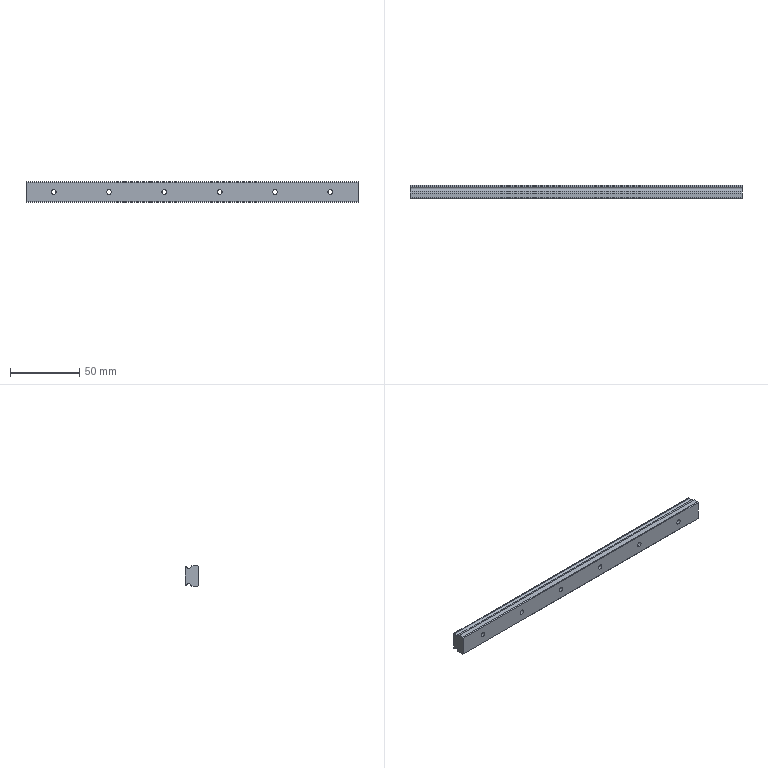Part | STEP file | RSR15M1V220201 Track^SRS15MUU-220LM-G10_Buffer motion shaft | 1 solid | 45 faces | box 240 x 9.5 x 15 mm | volume 30095 mm3 | cylinder 27 | plane 18 | commonest cylinder face diameters 3.5 x12 6 x12 3.18 x3